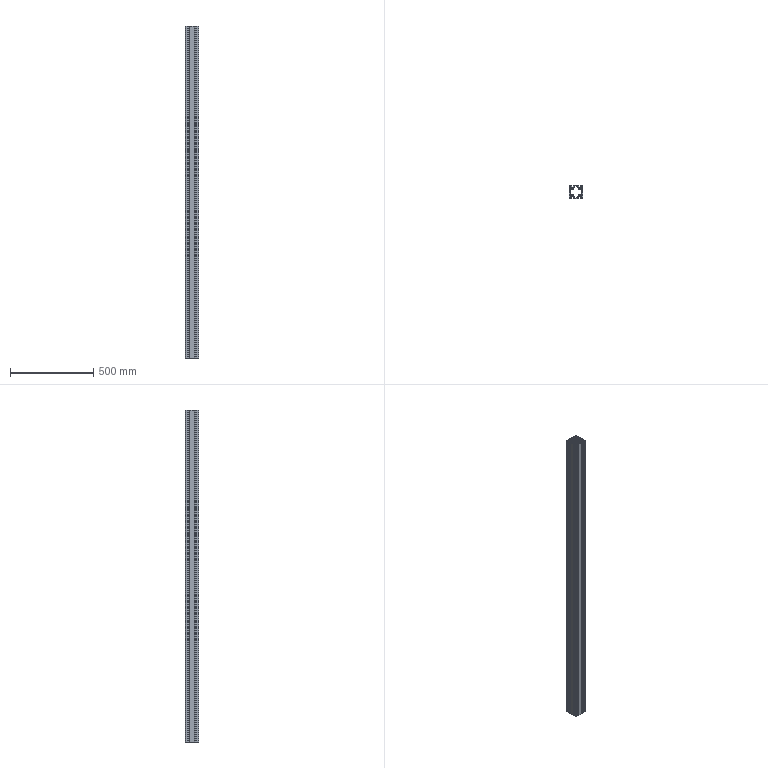Part | SolidWorks | features BaseBody 1 | 1 solid | 236 faces | box 80 x 80 x 1992 mm | volume 3392596 mm3 | plane 154 | cylinder 82 | commonest cylinder face diameters 2 x36 0.6 x20 6.8 x12 12 x10 6 x4